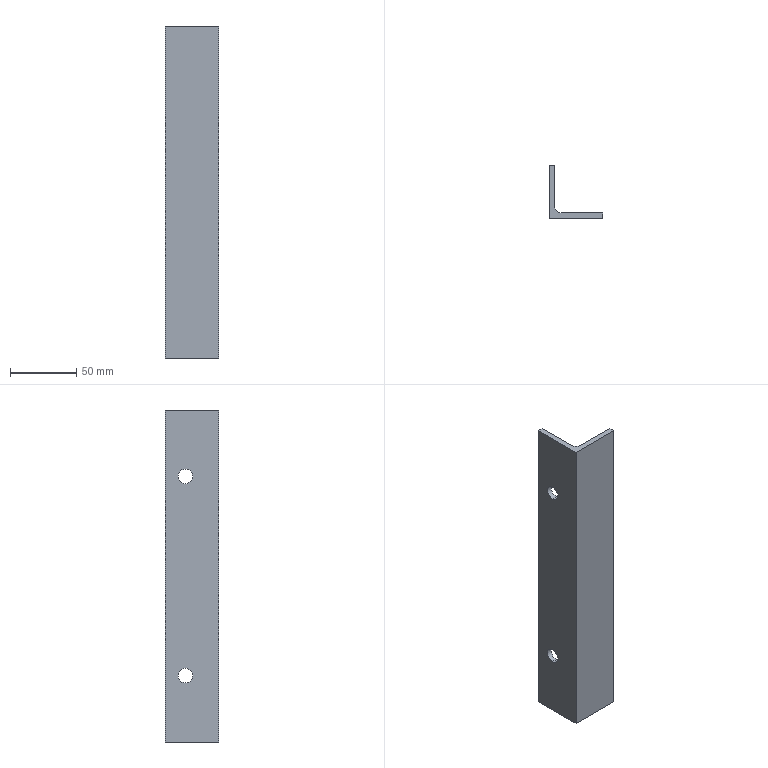Part | SolidWorks | features Extrusion 1, HoleWzd 1 | 1 solid | 15 faces | box 40 x 40 x 250 mm | volume 76581 mm3 | plane 8 | cylinder 7 | commonest cylinder face diameters 11 x4 0.02 x2 10 x1
STEP:
#1=CARTESIAN_POINT('',(4.,25.,194.5));
#2=VERTEX_POINT('',#1);
#3=CARTESIAN_POINT('',(4.,25.,205.5));
#4=VERTEX_POINT('',#3);
#5=CARTESIAN_POINT('',(4.,25.,200.));
#6=DIRECTION('',(-1.,0.,0.));
#7=DIRECTION('',(0.,-1.,0.));
#8=AXIS2_PLACEMENT_3D('',#5,#6,#7);
#9=CIRCLE('',#8,5.5);
#10=EDGE_CURVE('',#2,#4,#9,.T.);
#11=ORIENTED_EDGE('',*,*,#10,.F.);
#12=CARTESIAN_POINT('',(0.,25.,194.5));
#13=VERTEX_POINT('',#12);
#14=CARTESIAN_POINT('',(0.,25.,194.5));
#15=DIRECTION('',(-1.,0.,0.));
#16=VECTOR('',#15,1000.);
#17=LINE('',#14,#16);
#18=EDGE_CURVE('',#2,#13,#17,.T.);
#19=ORIENTED_EDGE('',*,*,#18,.T.);
#20=CARTESIAN_POINT('',(0.,25.,205.5));
#21=VERTEX_POINT('',#20);
#22=CARTESIAN_POINT('',(0.,25.,200.));
#23=DIRECTION('',(-1.,0.,0.));
#24=DIRECTION('',(0.,0.,1.));
#25=AXIS2_PLACEMENT_3D('',#22,#23,#24);
#26=CIRCLE('',#25,5.5);
#27=EDGE_CURVE('',#13,#21,#26,.T.);
#28=ORIENTED_EDGE('',*,*,#27,.T.);
#29=CARTESIAN_POINT('',(0.,25.,205.5));
#30=DIRECTION('',(-1.,0.,0.));
#31=VECTOR('',#30,1000.);
#32=LINE('',#29,#31);
#33=EDGE_CURVE('',#4,#21,#32,.T.);
#34=ORIENTED_EDGE('',*,*,#33,.F.);
#35=EDGE_LOOP('',(#11,#19,#28,#34));
#36=FACE_OUTER_BOUND('',#35,.T.);
#37=CARTESIAN_POINT('',(0.,25.,200.));
#38=DIRECTION('',(-1.,0.,0.));
#39=DIRECTION('',(0.,0.,1.));
#40=AXIS2_PLACEMENT_3D('',#37,#38,#39);
#41=CYLINDRICAL_SURFACE('',#40,5.5);
#42=ADVANCED_FACE('',(#36),#41,.F.);
#43=CARTESIAN_POINT('',(4.,25.,44.5));
#44=VERTEX_POINT('',#43);
#45=CARTESIAN_POINT('',(4.,25.,55.5));
#46=VERTEX_POINT('',#45);
#47=CARTESIAN_POINT('',(4.,25.,50.));
#48=DIRECTION('',(-1.,0.,0.));
#49=DIRECTION('',(0.,-1.,0.));
#50=AXIS2_PLACEMENT_3D('',#47,#48,#49);
#51=CIRCLE('',#50,5.5);
#52=EDGE_CURVE('',#44,#46,#51,.T.);
#53=ORIENTED_EDGE('',*,*,#52,.F.);
#54=CARTESIAN_POINT('',(0.,25.,44.5));
#55=VERTEX_POINT('',#54);
#56=CARTESIAN_POINT('',(0.,25.,44.5));
#57=DIRECTION('',(-1.,0.,0.));
#58=VECTOR('',#57,1000.);
#59=LINE('',#56,#58);
#60=EDGE_CURVE('',#44,#55,#59,.T.);
#61=ORIENTED_EDGE('',*,*,#60,.T.);
#62=CARTESIAN_POINT('',(0.,25.,55.5));
#63=VERTEX_POINT('',#62);
#64=CARTESIAN_POINT('',(0.,25.,50.));
#65=DIRECTION('',(-1.,0.,0.));
#66=DIRECTION('',(0.,0.,1.));
#67=AXIS2_PLACEMENT_3D('',#64,#65,#66);
#68=CIRCLE('',#67,5.5);
#69=EDGE_CURVE('',#55,#63,#68,.T.);
#70=ORIENTED_EDGE('',*,*,#69,.T.);
#71=CARTESIAN_POINT('',(0.,25.,55.5));
#72=DIRECTION('',(-1.,0.,0.));
#73=VECTOR('',#72,1000.);
#74=LINE('',#71,#73);
#75=EDGE_CURVE('',#46,#63,#74,.T.);
#76=ORIENTED_EDGE('',*,*,#75,.F.);
#77=EDGE_LOOP('',(#53,#61,#70,#76));
#78=FACE_OUTER_BOUND('',#77,.T.);
#79=CARTESIAN_POINT('',(0.,25.,50.));
#80=DIRECTION('',(-1.,0.,0.));
#81=DIRECTION('',(0.,0.,1.));
#82=AXIS2_PLACEMENT_3D('',#79,#80,#81);
#83=CYLINDRICAL_SURFACE('',#82,5.5);
#84=ADVANCED_FACE('',(#78),#83,.F.);
#85=CARTESIAN_POINT('',(0.,0.,0.));
#86=VERTEX_POINT('',#85);
#87=CARTESIAN_POINT('',(40.,0.,0.));
#88=VERTEX_POINT('',#87);
#89=CARTESIAN_POINT('',(40.,0.,0.));
#90=DIRECTION('',(1.,0.,0.));
#91=VECTOR('',#90,1000.);
#92=LINE('',#89,#91);
#93=EDGE_CURVE('',#86,#88,#92,.T.);
#94=ORIENTED_EDGE('',*,*,#93,.T.);
#95=CARTESIAN_POINT('',(40.,0.,250.));
#96=VERTEX_POINT('',#95);
#97=CARTESIAN_POINT('',(40.,0.,250.));
#98=DIRECTION('',(0.,0.,-1.));
#99=VECTOR('',#98,1000.);
#100=LINE('',#97,#99);
#101=EDGE_CURVE('',#96,#88,#100,.T.);
#102=ORIENTED_EDGE('',*,*,#101,.F.);
#103=CARTESIAN_POINT('',(0.,0.,250.));
#104=VERTEX_POINT('',#103);
#105=CARTESIAN_POINT('',(40.,0.,250.));
#106=DIRECTION('',(1.,0.,0.));
#107=VECTOR('',#106,1000.);
#108=LINE('',#105,#107);
#109=EDGE_CURVE('',#104,#96,#108,.T.);
#110=ORIENTED_EDGE('',*,*,#109,.F.);
#111=CARTESIAN_POINT('',(0.,0.,250.));
#112=DIRECTION('',(0.,0.,-1.));
#113=VECTOR('',#112,1000.);
#114=LINE('',#111,#113);
#115=EDGE_CURVE('',#104,#86,#114,.T.);
#116=ORIENTED_EDGE('',*,*,#115,.T.);
#117=EDGE_LOOP('',(#94,#102,#110,#116));
#118=FACE_OUTER_BOUND('',#117,.T.);
#119=CARTESIAN_POINT('',(40.,0.,250.));
#120=DIRECTION('',(0.,1.,0.));
#121=DIRECTION('',(-1.,0.,0.));
#122=AXIS2_PLACEMENT_3D('',#119,#120,#121);
#123=PLANE('',#122);
#124=ADVANCED_FACE('',(#118),#123,.F.);
#125=CARTESIAN_POINT('',(40.,3.99,0.));
#126=VERTEX_POINT('',#125);
#127=CARTESIAN_POINT('',(40.,3.99,0.));
#128=DIRECTION('',(0.,1.,0.));
#129=VECTOR('',#128,1000.);
#130=LINE('',#127,#129);
#131=EDGE_CURVE('',#88,#126,#130,.T.);
#132=ORIENTED_EDGE('',*,*,#131,.T.);
#133=CARTESIAN_POINT('',(40.,3.99,250.));
#134=VERTEX_POINT('',#133);
#135=CARTESIAN_POINT('',(40.,3.99,250.));
#136=DIRECTION('',(0.,0.,-1.));
#137=VECTOR('',#136,1000.);
#138=LINE('',#135,#137);
#139=EDGE_CURVE('',#134,#126,#138,.T.);
#140=ORIENTED_EDGE('',*,*,#139,.F.);
#141=CARTESIAN_POINT('',(40.,3.99,250.));
#142=DIRECTION('',(0.,1.,0.));
#143=VECTOR('',#142,1000.);
#144=LINE('',#141,#143);
#145=EDGE_CURVE('',#96,#134,#144,.T.);
#146=ORIENTED_EDGE('',*,*,#145,.F.);
#147=ORIENTED_EDGE('',*,*,#101,.T.);
#148=EDGE_LOOP('',(#132,#140,#146,#147));
#149=FACE_OUTER_BOUND('',#148,.T.);
#150=CARTESIAN_POINT('',(40.,3.99,250.));
#151=DIRECTION('',(-1.,0.,0.));
#152=DIRECTION('',(0.,0.,1.));
#153=AXIS2_PLACEMENT_3D('',#150,#151,#152);
#154=PLANE('',#153);
#155=ADVANCED_FACE('',(#149),#154,.F.);
#156=CARTESIAN_POINT('',(39.99,4.,0.));
#157=VERTEX_POINT('',#156);
#158=CARTESIAN_POINT('',(39.99,3.99,0.));
#159=DIRECTION('',(0.,0.,1.));
#160=DIRECTION('',(1.,0.,0.));
#161=AXIS2_PLACEMENT_3D('',#158,#159,#160);
#162=CIRCLE('',#161,0.01);
#163=EDGE_CURVE('',#126,#157,#162,.T.);
#164=ORIENTED_EDGE('',*,*,#163,.T.);
#165=CARTESIAN_POINT('',(39.99,4.,250.));
#166=VERTEX_POINT('',#165);
#167=CARTESIAN_POINT('',(39.99,4.,250.));
#168=DIRECTION('',(0.,0.,-1.));
#169=VECTOR('',#168,1000.);
#170=LINE('',#167,#169);
#171=EDGE_CURVE('',#166,#157,#170,.T.);
#172=ORIENTED_EDGE('',*,*,#171,.F.);
#173=CARTESIAN_POINT('',(39.99,3.99,250.));
#174=DIRECTION('',(0.,0.,1.));
#175=DIRECTION('',(1.,0.,0.));
#176=AXIS2_PLACEMENT_3D('',#173,#174,#175);
#177=CIRCLE('',#176,0.01);
#178=EDGE_CURVE('',#134,#166,#177,.T.);
#179=ORIENTED_EDGE('',*,*,#178,.F.);
#180=ORIENTED_EDGE('',*,*,#139,.T.);
#181=EDGE_LOOP('',(#164,#172,#179,#180));
#182=FACE_OUTER_BOUND('',#181,.T.);
#183=CARTESIAN_POINT('',(39.99,3.99,250.));
#184=DIRECTION('',(0.,0.,-1.));
#185=DIRECTION('',(-1.,0.,0.));
#186=AXIS2_PLACEMENT_3D('',#183,#184,#185);
#187=CYLINDRICAL_SURFACE('',#186,0.01);
#188=ADVANCED_FACE('',(#182),#187,.T.);
#189=CARTESIAN_POINT('',(9.,4.,0.));
#190=VERTEX_POINT('',#189);
#191=CARTESIAN_POINT('',(9.,4.,0.));
#192=DIRECTION('',(-1.,0.,0.));
#193=VECTOR('',#192,1000.);
#194=LINE('',#191,#193);
#195=EDGE_CURVE('',#157,#190,#194,.T.);
#196=ORIENTED_EDGE('',*,*,#195,.T.);
#197=CARTESIAN_POINT('',(9.,4.,250.));
#198=VERTEX_POINT('',#197);
#199=CARTESIAN_POINT('',(9.,4.,250.));
#200=DIRECTION('',(0.,0.,-1.));
#201=VECTOR('',#200,1000.);
#202=LINE('',#199,#201);
#203=EDGE_CURVE('',#198,#190,#202,.T.);
#204=ORIENTED_EDGE('',*,*,#203,.F.);
#205=CARTESIAN_POINT('',(9.,4.,250.));
#206=DIRECTION('',(-1.,0.,0.));
#207=VECTOR('',#206,1000.);
#208=LINE('',#205,#207);
#209=EDGE_CURVE('',#166,#198,#208,.T.);
#210=ORIENTED_EDGE('',*,*,#209,.F.);
#211=ORIENTED_EDGE('',*,*,#171,.T.);
#212=EDGE_LOOP('',(#196,#204,#210,#211));
#213=FACE_OUTER_BOUND('',#212,.T.);
#214=CARTESIAN_POINT('',(9.,4.,250.));
#215=DIRECTION('',(0.,-1.,0.));
#216=DIRECTION('',(0.,0.,-1.));
#217=AXIS2_PLACEMENT_3D('',#214,#215,#216);
#218=PLANE('',#217);
#219=ADVANCED_FACE('',(#213),#218,.F.);
#220=CARTESIAN_POINT('',(4.,9.,0.));
#221=VERTEX_POINT('',#220);
#222=CARTESIAN_POINT('',(9.,9.,0.));
#223=DIRECTION('',(0.,0.,-1.));
#224=DIRECTION('',(-1.,0.,0.));
#225=AXIS2_PLACEMENT_3D('',#222,#223,#224);
#226=CIRCLE('',#225,5.);
#227=EDGE_CURVE('',#190,#221,#226,.T.);
#228=ORIENTED_EDGE('',*,*,#227,.T.);
#229=CARTESIAN_POINT('',(4.,9.,250.));
#230=VERTEX_POINT('',#229);
#231=CARTESIAN_POINT('',(4.,9.,250.));
#232=DIRECTION('',(0.,0.,-1.));
#233=VECTOR('',#232,1000.);
#234=LINE('',#231,#233);
#235=EDGE_CURVE('',#230,#221,#234,.T.);
#236=ORIENTED_EDGE('',*,*,#235,.F.);
#237=CARTESIAN_POINT('',(9.,9.,250.));
#238=DIRECTION('',(0.,0.,-1.));
#239=DIRECTION('',(-1.,0.,0.));
#240=AXIS2_PLACEMENT_3D('',#237,#238,#239);
#241=CIRCLE('',#240,5.);
#242=EDGE_CURVE('',#198,#230,#241,.T.);
#243=ORIENTED_EDGE('',*,*,#242,.F.);
#244=ORIENTED_EDGE('',*,*,#203,.T.);
#245=EDGE_LOOP('',(#228,#236,#243,#244));
#246=FACE_OUTER_BOUND('',#245,.T.);
#247=CARTESIAN_POINT('',(9.,9.,250.));
#248=DIRECTION('',(0.,0.,-1.));
#249=DIRECTION('',(-1.,0.,0.));
#250=AXIS2_PLACEMENT_3D('',#247,#248,#249);
#251=CYLINDRICAL_SURFACE('',#250,5.);
#252=ADVANCED_FACE('',(#246),#251,.F.);
#253=CARTESIAN_POINT('',(4.,25.,200.));
#254=DIRECTION('',(-1.,0.,0.));
#255=DIRECTION('',(0.,-1.,0.));
#256=AXIS2_PLACEMENT_3D('',#253,#254,#255);
#257=CIRCLE('',#256,5.5);
#258=EDGE_CURVE('',#4,#2,#257,.T.);
#259=ORIENTED_EDGE('',*,*,#258,.T.);
#260=ORIENTED_EDGE('',*,*,#10,.T.);
#261=EDGE_LOOP('',(#259,#260));
#262=FACE_BOUND('',#261,.T.);
#263=CARTESIAN_POINT('',(4.,25.,50.));
#264=DIRECTION('',(-1.,0.,0.));
#265=DIRECTION('',(0.,-1.,0.));
#266=AXIS2_PLACEMENT_3D('',#263,#264,#265);
#267=CIRCLE('',#266,5.5);
#268=EDGE_CURVE('',#46,#44,#267,.T.);
#269=ORIENTED_EDGE('',*,*,#268,.T.);
#270=ORIENTED_EDGE('',*,*,#52,.T.);
#271=EDGE_LOOP('',(#269,#270));
#272=FACE_BOUND('',#271,.T.);
#273=CARTESIAN_POINT('',(4.,39.99,0.));
#274=VERTEX_POINT('',#273);
#275=CARTESIAN_POINT('',(4.,39.99,0.));
#276=DIRECTION('',(0.,1.,0.));
#277=VECTOR('',#276,1000.);
#278=LINE('',#275,#277);
#279=EDGE_CURVE('',#221,#274,#278,.T.);
#280=ORIENTED_EDGE('',*,*,#279,.T.);
#281=CARTESIAN_POINT('',(4.,39.99,250.));
#282=VERTEX_POINT('',#281);
#283=CARTESIAN_POINT('',(4.,39.99,250.));
#284=DIRECTION('',(0.,0.,-1.));
#285=VECTOR('',#284,1000.);
#286=LINE('',#283,#285);
#287=EDGE_CURVE('',#282,#274,#286,.T.);
#288=ORIENTED_EDGE('',*,*,#287,.F.);
#289=CARTESIAN_POINT('',(4.,39.99,250.));
#290=DIRECTION('',(0.,1.,0.));
#291=VECTOR('',#290,1000.);
#292=LINE('',#289,#291);
#293=EDGE_CURVE('',#230,#282,#292,.T.);
#294=ORIENTED_EDGE('',*,*,#293,.F.);
#295=ORIENTED_EDGE('',*,*,#235,.T.);
#296=EDGE_LOOP('',(#280,#288,#294,#295));
#297=FACE_OUTER_BOUND('',#296,.T.);
#298=CARTESIAN_POINT('',(4.,39.99,250.));
#299=DIRECTION('',(-1.,0.,0.));
#300=DIRECTION('',(0.,-1.,0.));
#301=AXIS2_PLACEMENT_3D('',#298,#299,#300);
#302=PLANE('',#301);
#303=ADVANCED_FACE('',(#262,#272,#297),#302,.F.);
#304=CARTESIAN_POINT('',(3.99,40.,0.));
#305=VERTEX_POINT('',#304);
#306=CARTESIAN_POINT('',(3.99,39.99,0.));
#307=DIRECTION('',(0.,0.,1.));
#308=DIRECTION('',(1.,0.,0.));
#309=AXIS2_PLACEMENT_3D('',#306,#307,#308);
#310=CIRCLE('',#309,0.01);
#311=EDGE_CURVE('',#274,#305,#310,.T.);
#312=ORIENTED_EDGE('',*,*,#311,.T.);
#313=CARTESIAN_POINT('',(3.99,40.,250.));
#314=VERTEX_POINT('',#313);
#315=CARTESIAN_POINT('',(3.99,40.,250.));
#316=DIRECTION('',(0.,0.,-1.));
#317=VECTOR('',#316,1000.);
#318=LINE('',#315,#317);
#319=EDGE_CURVE('',#314,#305,#318,.T.);
#320=ORIENTED_EDGE('',*,*,#319,.F.);
#321=CARTESIAN_POINT('',(3.99,39.99,250.));
#322=DIRECTION('',(0.,0.,1.));
#323=DIRECTION('',(1.,0.,0.));
#324=AXIS2_PLACEMENT_3D('',#321,#322,#323);
#325=CIRCLE('',#324,0.01);
#326=EDGE_CURVE('',#282,#314,#325,.T.);
#327=ORIENTED_EDGE('',*,*,#326,.F.);
#328=ORIENTED_EDGE('',*,*,#287,.T.);
#329=EDGE_LOOP('',(#312,#320,#327,#328));
#330=FACE_OUTER_BOUND('',#329,.T.);
#331=CARTESIAN_POINT('',(3.99,39.99,250.));
#332=DIRECTION('',(0.,0.,-1.));
#333=DIRECTION('',(-1.,0.,0.));
#334=AXIS2_PLACEMENT_3D('',#331,#332,#333);
#335=CYLINDRICAL_SURFACE('',#334,0.01);
#336=ADVANCED_FACE('',(#330),#335,.T.);
#337=CARTESIAN_POINT('',(0.,40.,0.));
#338=VERTEX_POINT('',#337);
#339=CARTESIAN_POINT('',(0.,40.,0.));
#340=DIRECTION('',(-1.,0.,0.));
#341=VECTOR('',#340,1000.);
#342=LINE('',#339,#341);
#343=EDGE_CURVE('',#305,#338,#342,.T.);
#344=ORIENTED_EDGE('',*,*,#343,.T.);
#345=CARTESIAN_POINT('',(0.,40.,250.));
#346=VERTEX_POINT('',#345);
#347=CARTESIAN_POINT('',(0.,40.,250.));
#348=DIRECTION('',(0.,0.,-1.));
#349=VECTOR('',#348,1000.);
#350=LINE('',#347,#349);
#351=EDGE_CURVE('',#346,#338,#350,.T.);
#352=ORIENTED_EDGE('',*,*,#351,.F.);
#353=CARTESIAN_POINT('',(0.,40.,250.));
#354=DIRECTION('',(-1.,0.,0.));
#355=VECTOR('',#354,1000.);
#356=LINE('',#353,#355);
#357=EDGE_CURVE('',#314,#346,#356,.T.);
#358=ORIENTED_EDGE('',*,*,#357,.F.);
#359=ORIENTED_EDGE('',*,*,#319,.T.);
#360=EDGE_LOOP('',(#344,#352,#358,#359));
#361=FACE_OUTER_BOUND('',#360,.T.);
#362=CARTESIAN_POINT('',(0.,40.,250.));
#363=DIRECTION('',(0.,-1.,0.));
#364=DIRECTION('',(0.,0.,-1.));
#365=AXIS2_PLACEMENT_3D('',#362,#363,#364);
#366=PLANE('',#365);
#367=ADVANCED_FACE('',(#361),#366,.F.);
#368=CARTESIAN_POINT('',(0.,25.,200.));
#369=DIRECTION('',(-1.,0.,0.));
#370=DIRECTION('',(0.,0.,1.));
#371=AXIS2_PLACEMENT_3D('',#368,#369,#370);
#372=CIRCLE('',#371,5.5);
#373=EDGE_CURVE('',#21,#13,#372,.T.);
#374=ORIENTED_EDGE('',*,*,#373,.F.);
#375=ORIENTED_EDGE('',*,*,#27,.F.);
#376=EDGE_LOOP('',(#374,#375));
#377=FACE_BOUND('',#376,.T.);
#378=CARTESIAN_POINT('',(0.,25.,50.));
#379=DIRECTION('',(-1.,0.,0.));
#380=DIRECTION('',(0.,0.,1.));
#381=AXIS2_PLACEMENT_3D('',#378,#379,#380);
#382=CIRCLE('',#381,5.5);
#383=EDGE_CURVE('',#63,#55,#382,.T.);
#384=ORIENTED_EDGE('',*,*,#383,.F.);
#385=ORIENTED_EDGE('',*,*,#69,.F.);
#386=EDGE_LOOP('',(#384,#385));
#387=FACE_BOUND('',#386,.T.);
#388=CARTESIAN_POINT('',(0.,0.,0.));
#389=DIRECTION('',(0.,-1.,0.));
#390=VECTOR('',#389,1000.);
#391=LINE('',#388,#390);
#392=EDGE_CURVE('',#338,#86,#391,.T.);
#393=ORIENTED_EDGE('',*,*,#392,.T.);
#394=ORIENTED_EDGE('',*,*,#115,.F.);
#395=CARTESIAN_POINT('',(0.,0.,250.));
#396=DIRECTION('',(0.,-1.,0.));
#397=VECTOR('',#396,1000.);
#398=LINE('',#395,#397);
#399=EDGE_CURVE('',#346,#104,#398,.T.);
#400=ORIENTED_EDGE('',*,*,#399,.F.);
#401=ORIENTED_EDGE('',*,*,#351,.T.);
#402=EDGE_LOOP('',(#393,#394,#400,#401));
#403=FACE_OUTER_BOUND('',#402,.T.);
#404=CARTESIAN_POINT('',(0.,0.,250.));
#405=DIRECTION('',(1.,0.,0.));
#406=DIRECTION('',(0.,0.,-1.));
#407=AXIS2_PLACEMENT_3D('',#404,#405,#406);
#408=PLANE('',#407);
#409=ADVANCED_FACE('',(#377,#387,#403),#408,.F.);
#410=ORIENTED_EDGE('',*,*,#109,.T.);
#411=ORIENTED_EDGE('',*,*,#145,.T.);
#412=ORIENTED_EDGE('',*,*,#178,.T.);
#413=ORIENTED_EDGE('',*,*,#209,.T.);
#414=ORIENTED_EDGE('',*,*,#242,.T.);
#415=ORIENTED_EDGE('',*,*,#293,.T.);
#416=ORIENTED_EDGE('',*,*,#326,.T.);
#417=ORIENTED_EDGE('',*,*,#357,.T.);
#418=ORIENTED_EDGE('',*,*,#399,.T.);
#419=EDGE_LOOP('',(#410,#411,#412,#413,#414,#415,#416,#417,#418));
#420=FACE_OUTER_BOUND('',#419,.T.);
#421=CARTESIAN_POINT('',(3.99,39.99,250.));
#422=DIRECTION('',(0.,0.,1.));
#423=DIRECTION('',(1.,0.,0.));
#424=AXIS2_PLACEMENT_3D('',#421,#422,#423);
#425=PLANE('',#424);
#426=ADVANCED_FACE('',(#420),#425,.T.);
#427=ORIENTED_EDGE('',*,*,#93,.F.);
#428=ORIENTED_EDGE('',*,*,#392,.F.);
#429=ORIENTED_EDGE('',*,*,#343,.F.);
#430=ORIENTED_EDGE('',*,*,#311,.F.);
#431=ORIENTED_EDGE('',*,*,#279,.F.);
#432=ORIENTED_EDGE('',*,*,#227,.F.);
#433=ORIENTED_EDGE('',*,*,#195,.F.);
#434=ORIENTED_EDGE('',*,*,#163,.F.);
#435=ORIENTED_EDGE('',*,*,#131,.F.);
#436=EDGE_LOOP('',(#427,#428,#429,#430,#431,#432,#433,#434,#435));
#437=FACE_OUTER_BOUND('',#436,.T.);
#438=CARTESIAN_POINT('',(3.99,39.99,0.));
#439=DIRECTION('',(0.,0.,1.));
#440=DIRECTION('',(1.,0.,0.));
#441=AXIS2_PLACEMENT_3D('',#438,#439,#440);
#442=PLANE('',#441);
#443=ADVANCED_FACE('',(#437),#442,.F.);
#444=ORIENTED_EDGE('',*,*,#60,.F.);
#445=ORIENTED_EDGE('',*,*,#268,.F.);
#446=ORIENTED_EDGE('',*,*,#75,.T.);
#447=ORIENTED_EDGE('',*,*,#383,.T.);
#448=EDGE_LOOP('',(#444,#445,#446,#447));
#449=FACE_OUTER_BOUND('',#448,.T.);
#450=CARTESIAN_POINT('',(0.,25.,50.));
#451=DIRECTION('',(-1.,0.,0.));
#452=DIRECTION('',(0.,0.,1.));
#453=AXIS2_PLACEMENT_3D('',#450,#451,#452);
#454=CYLINDRICAL_SURFACE('',#453,5.5);
#455=ADVANCED_FACE('',(#449),#454,.F.);
#456=ORIENTED_EDGE('',*,*,#18,.F.);
#457=ORIENTED_EDGE('',*,*,#258,.F.);
#458=ORIENTED_EDGE('',*,*,#33,.T.);
#459=ORIENTED_EDGE('',*,*,#373,.T.);
#460=EDGE_LOOP('',(#456,#457,#458,#459));
#461=FACE_OUTER_BOUND('',#460,.T.);
#462=CARTESIAN_POINT('',(0.,25.,200.));
#463=DIRECTION('',(-1.,0.,0.));
#464=DIRECTION('',(0.,0.,1.));
#465=AXIS2_PLACEMENT_3D('',#462,#463,#464);
#466=CYLINDRICAL_SURFACE('',#465,5.5);
#467=ADVANCED_FACE('',(#461),#466,.F.);
#468=CLOSED_SHELL('',(#42,#84,#124,#155,#188,#219,#252,#303,#336,#367,#409,#426,#443,#455,#467));
#469=MANIFOLD_SOLID_BREP('',#468);
#470=CARTESIAN_POINT('',(0.,0.,0.));
#471=DIRECTION('',(0.,0.,1.));
#472=DIRECTION('',(1.,0.,0.));
#473=AXIS2_PLACEMENT_3D('',#470,#471,#472);
#474=(LENGTH_UNIT()NAMED_UNIT(*)SI_UNIT(.MILLI.,.METRE.));
#475=UNCERTAINTY_MEASURE_WITH_UNIT(LENGTH_MEASURE(0.00001),#474,'','');
#476=(NAMED_UNIT(*)PLANE_ANGLE_UNIT()SI_UNIT($,.RADIAN.));
#477=(NAMED_UNIT(*)SI_UNIT($,.STERADIAN.)SOLID_ANGLE_UNIT());
#478=(GEOMETRIC_REPRESENTATION_CONTEXT(3)GLOBAL_UNCERTAINTY_ASSIGNED_CONTEXT((#475))GLOBAL_UNIT_ASSIGNED_CONTEXT((#474,#476,#477))REPRESENTATION_CONTEXT('',''));
#479=ADVANCED_BREP_SHAPE_REPRESENTATION('',(#469,#473),#478);